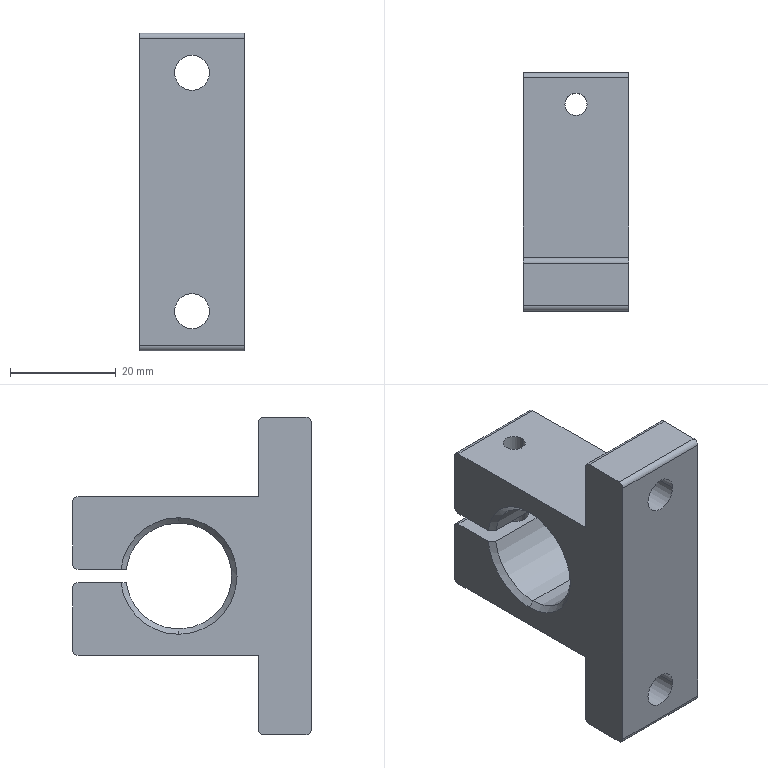Part | STEP file | Guide shaft support SHAT-2025 | 1 solid | 41 faces | box 20 x 45 x 60 mm | volume 24589 mm3 | cylinder 21 | plane 14 | cone 6 | commonest cylinder face diameters 2 x8 6.6 x4 20 x3 4.2 x2 5.5 x2 10 x2